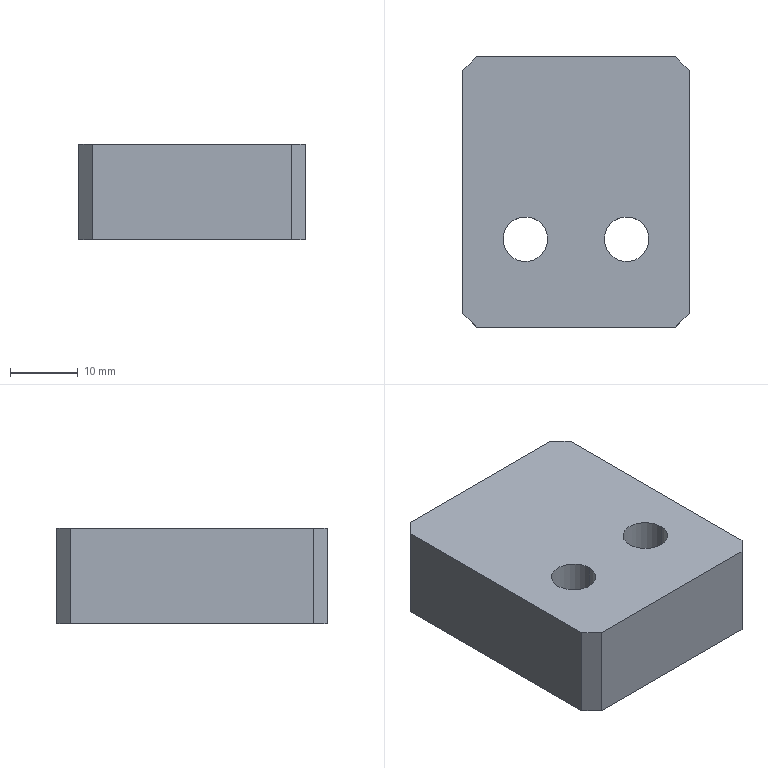Part | NX | features BREP 1 | 1 solid | 28 faces | box 33.5 x 40 x 14.15 mm | volume 16795 mm3 | cylinder 12 | plane 12 | cone 4 | commonest cylinder face diameters 4.2 x4 6.6 x4 11 x4
STEP:
#1=CARTESIAN_POINT('',(14.,-31.,6.));
#2=VERTEX_POINT('',#1);
#3=CARTESIAN_POINT('',(3.,-31.,6.));
#4=VERTEX_POINT('',#3);
#5=CARTESIAN_POINT('',(8.5,-31.,6.));
#6=DIRECTION('',(0.,0.,-1.));
#7=DIRECTION('',(-1.,0.,0.));
#8=AXIS2_PLACEMENT_3D('',#5,#6,#7);
#9=CIRCLE('',#8,5.5);
#10=EDGE_CURVE('',#2,#4,#9,.T.);
#11=ORIENTED_EDGE('',*,*,#10,.F.);
#12=CARTESIAN_POINT('',(14.,-31.,0.));
#13=VERTEX_POINT('',#12);
#14=CARTESIAN_POINT('',(14.,-31.,0.));
#15=DIRECTION('',(0.,0.,-1.));
#16=VECTOR('',#15,1000.);
#17=LINE('',#14,#16);
#18=EDGE_CURVE('',#2,#13,#17,.T.);
#19=ORIENTED_EDGE('',*,*,#18,.T.);
#20=CARTESIAN_POINT('',(3.,-31.,0.));
#21=VERTEX_POINT('',#20);
#22=CARTESIAN_POINT('',(8.5,-31.,0.));
#23=DIRECTION('',(0.,0.,-1.));
#24=DIRECTION('',(-1.,0.,0.));
#25=AXIS2_PLACEMENT_3D('',#22,#23,#24);
#26=CIRCLE('',#25,5.5);
#27=EDGE_CURVE('',#13,#21,#26,.T.);
#28=ORIENTED_EDGE('',*,*,#27,.T.);
#29=CARTESIAN_POINT('',(3.,-31.,0.));
#30=DIRECTION('',(0.,0.,-1.));
#31=VECTOR('',#30,1000.);
#32=LINE('',#29,#31);
#33=EDGE_CURVE('',#4,#21,#32,.T.);
#34=ORIENTED_EDGE('',*,*,#33,.F.);
#35=EDGE_LOOP('',(#11,#19,#28,#34));
#36=FACE_BOUND('',#35,.T.);
#37=CARTESIAN_POINT('',(8.5,-31.,0.));
#38=DIRECTION('',(0.,0.,-1.));
#39=DIRECTION('',(-1.,0.,0.));
#40=AXIS2_PLACEMENT_3D('',#37,#38,#39);
#41=CYLINDRICAL_SURFACE('',#40,5.5);
#42=ADVANCED_FACE('',(#36),#41,.F.);
#43=CARTESIAN_POINT('',(11.8,-31.,14.15));
#44=VERTEX_POINT('',#43);
#45=CARTESIAN_POINT('',(5.2,-31.,14.15));
#46=VERTEX_POINT('',#45);
#47=CARTESIAN_POINT('',(8.5,-31.,14.15));
#48=DIRECTION('',(0.,0.,-1.));
#49=DIRECTION('',(-1.,0.,0.));
#50=AXIS2_PLACEMENT_3D('',#47,#48,#49);
#51=CIRCLE('',#50,3.3);
#52=EDGE_CURVE('',#44,#46,#51,.T.);
#53=ORIENTED_EDGE('',*,*,#52,.F.);
#54=CARTESIAN_POINT('',(11.8,-31.,6.));
#55=VERTEX_POINT('',#54);
#56=CARTESIAN_POINT('',(11.8,-31.,0.));
#57=DIRECTION('',(0.,0.,-1.));
#58=VECTOR('',#57,1000.);
#59=LINE('',#56,#58);
#60=EDGE_CURVE('',#44,#55,#59,.T.);
#61=ORIENTED_EDGE('',*,*,#60,.T.);
#62=CARTESIAN_POINT('',(5.2,-31.,6.));
#63=VERTEX_POINT('',#62);
#64=CARTESIAN_POINT('',(8.5,-31.,6.));
#65=DIRECTION('',(0.,0.,-1.));
#66=DIRECTION('',(-1.,0.,0.));
#67=AXIS2_PLACEMENT_3D('',#64,#65,#66);
#68=CIRCLE('',#67,3.3);
#69=EDGE_CURVE('',#55,#63,#68,.T.);
#70=ORIENTED_EDGE('',*,*,#69,.T.);
#71=CARTESIAN_POINT('',(5.2,-31.,0.));
#72=DIRECTION('',(0.,0.,-1.));
#73=VECTOR('',#72,1000.);
#74=LINE('',#71,#73);
#75=EDGE_CURVE('',#46,#63,#74,.T.);
#76=ORIENTED_EDGE('',*,*,#75,.F.);
#77=EDGE_LOOP('',(#53,#61,#70,#76));
#78=FACE_BOUND('',#77,.T.);
#79=CARTESIAN_POINT('',(8.5,-31.,0.));
#80=DIRECTION('',(0.,0.,-1.));
#81=DIRECTION('',(-1.,0.,0.));
#82=AXIS2_PLACEMENT_3D('',#79,#80,#81);
#83=CYLINDRICAL_SURFACE('',#82,3.3);
#84=ADVANCED_FACE('',(#78),#83,.F.);
#85=CARTESIAN_POINT('',(-1.,-31.,6.));
#86=VERTEX_POINT('',#85);
#87=CARTESIAN_POINT('',(-12.,-31.,6.));
#88=VERTEX_POINT('',#87);
#89=CARTESIAN_POINT('',(-6.5,-31.,6.));
#90=DIRECTION('',(0.,0.,-1.));
#91=DIRECTION('',(-1.,0.,0.));
#92=AXIS2_PLACEMENT_3D('',#89,#90,#91);
#93=CIRCLE('',#92,5.5);
#94=EDGE_CURVE('',#86,#88,#93,.T.);
#95=ORIENTED_EDGE('',*,*,#94,.F.);
#96=CARTESIAN_POINT('',(-1.,-31.,0.));
#97=VERTEX_POINT('',#96);
#98=CARTESIAN_POINT('',(-1.,-31.,0.));
#99=DIRECTION('',(0.,0.,-1.));
#100=VECTOR('',#99,1000.);
#101=LINE('',#98,#100);
#102=EDGE_CURVE('',#86,#97,#101,.T.);
#103=ORIENTED_EDGE('',*,*,#102,.T.);
#104=CARTESIAN_POINT('',(-12.,-31.,0.));
#105=VERTEX_POINT('',#104);
#106=CARTESIAN_POINT('',(-6.5,-31.,0.));
#107=DIRECTION('',(0.,0.,-1.));
#108=DIRECTION('',(-1.,0.,0.));
#109=AXIS2_PLACEMENT_3D('',#106,#107,#108);
#110=CIRCLE('',#109,5.5);
#111=EDGE_CURVE('',#97,#105,#110,.T.);
#112=ORIENTED_EDGE('',*,*,#111,.T.);
#113=CARTESIAN_POINT('',(-12.,-31.,0.));
#114=DIRECTION('',(0.,0.,-1.));
#115=VECTOR('',#114,1000.);
#116=LINE('',#113,#115);
#117=EDGE_CURVE('',#88,#105,#116,.T.);
#118=ORIENTED_EDGE('',*,*,#117,.F.);
#119=EDGE_LOOP('',(#95,#103,#112,#118));
#120=FACE_BOUND('',#119,.T.);
#121=CARTESIAN_POINT('',(-6.5,-31.,0.));
#122=DIRECTION('',(0.,0.,-1.));
#123=DIRECTION('',(-1.,0.,0.));
#124=AXIS2_PLACEMENT_3D('',#121,#122,#123);
#125=CYLINDRICAL_SURFACE('',#124,5.5);
#126=ADVANCED_FACE('',(#120),#125,.F.);
#127=CARTESIAN_POINT('',(-3.2,-31.,14.15));
#128=VERTEX_POINT('',#127);
#129=CARTESIAN_POINT('',(-9.8,-31.,14.15));
#130=VERTEX_POINT('',#129);
#131=CARTESIAN_POINT('',(-6.5,-31.,14.15));
#132=DIRECTION('',(0.,0.,-1.));
#133=DIRECTION('',(-1.,0.,0.));
#134=AXIS2_PLACEMENT_3D('',#131,#132,#133);
#135=CIRCLE('',#134,3.3);
#136=EDGE_CURVE('',#128,#130,#135,.T.);
#137=ORIENTED_EDGE('',*,*,#136,.F.);
#138=CARTESIAN_POINT('',(-3.2,-31.,6.));
#139=VERTEX_POINT('',#138);
#140=CARTESIAN_POINT('',(-3.2,-31.,0.));
#141=DIRECTION('',(0.,0.,-1.));
#142=VECTOR('',#141,1000.);
#143=LINE('',#140,#142);
#144=EDGE_CURVE('',#128,#139,#143,.T.);
#145=ORIENTED_EDGE('',*,*,#144,.T.);
#146=CARTESIAN_POINT('',(-9.8,-31.,6.));
#147=VERTEX_POINT('',#146);
#148=CARTESIAN_POINT('',(-6.5,-31.,6.));
#149=DIRECTION('',(0.,0.,-1.));
#150=DIRECTION('',(-1.,0.,0.));
#151=AXIS2_PLACEMENT_3D('',#148,#149,#150);
#152=CIRCLE('',#151,3.3);
#153=EDGE_CURVE('',#139,#147,#152,.T.);
#154=ORIENTED_EDGE('',*,*,#153,.T.);
#155=CARTESIAN_POINT('',(-9.8,-31.,0.));
#156=DIRECTION('',(0.,0.,-1.));
#157=VECTOR('',#156,1000.);
#158=LINE('',#155,#157);
#159=EDGE_CURVE('',#130,#147,#158,.T.);
#160=ORIENTED_EDGE('',*,*,#159,.F.);
#161=EDGE_LOOP('',(#137,#145,#154,#160));
#162=FACE_BOUND('',#161,.T.);
#163=CARTESIAN_POINT('',(-6.5,-31.,0.));
#164=DIRECTION('',(0.,0.,-1.));
#165=DIRECTION('',(-1.,0.,0.));
#166=AXIS2_PLACEMENT_3D('',#163,#164,#165);
#167=CYLINDRICAL_SURFACE('',#166,3.3);
#168=ADVANCED_FACE('',(#162),#167,.F.);
#169=CARTESIAN_POINT('',(13.6,-16.,12.4));
#170=VERTEX_POINT('',#169);
#171=CARTESIAN_POINT('',(9.4,-16.,12.4));
#172=VERTEX_POINT('',#171);
#173=CARTESIAN_POINT('',(11.5,-16.,12.4));
#174=DIRECTION('',(0.,0.,-1.));
#175=DIRECTION('',(-1.,0.,0.));
#176=AXIS2_PLACEMENT_3D('',#173,#174,#175);
#177=CIRCLE('',#176,2.1);
#178=EDGE_CURVE('',#170,#172,#177,.T.);
#179=ORIENTED_EDGE('',*,*,#178,.F.);
#180=CARTESIAN_POINT('',(13.6,-16.,0.));
#181=VERTEX_POINT('',#180);
#182=CARTESIAN_POINT('',(13.6,-16.,0.));
#183=DIRECTION('',(0.,0.,-1.));
#184=VECTOR('',#183,1000.);
#185=LINE('',#182,#184);
#186=EDGE_CURVE('',#170,#181,#185,.T.);
#187=ORIENTED_EDGE('',*,*,#186,.T.);
#188=CARTESIAN_POINT('',(9.4,-16.,0.));
#189=VERTEX_POINT('',#188);
#190=CARTESIAN_POINT('',(11.5,-16.,0.));
#191=DIRECTION('',(0.,0.,-1.));
#192=DIRECTION('',(-1.,0.,0.));
#193=AXIS2_PLACEMENT_3D('',#190,#191,#192);
#194=CIRCLE('',#193,2.1);
#195=EDGE_CURVE('',#181,#189,#194,.T.);
#196=ORIENTED_EDGE('',*,*,#195,.T.);
#197=CARTESIAN_POINT('',(9.4,-16.,0.));
#198=DIRECTION('',(0.,0.,-1.));
#199=VECTOR('',#198,1000.);
#200=LINE('',#197,#199);
#201=EDGE_CURVE('',#172,#189,#200,.T.);
#202=ORIENTED_EDGE('',*,*,#201,.F.);
#203=EDGE_LOOP('',(#179,#187,#196,#202));
#204=FACE_BOUND('',#203,.T.);
#205=CARTESIAN_POINT('',(11.5,-16.,0.));
#206=DIRECTION('',(0.,0.,-1.));
#207=DIRECTION('',(-1.,0.,0.));
#208=AXIS2_PLACEMENT_3D('',#205,#206,#207);
#209=CYLINDRICAL_SURFACE('',#208,2.1);
#210=ADVANCED_FACE('',(#204),#209,.F.);
#211=CARTESIAN_POINT('',(11.5,-16.,13.662));
#212=VERTEX_POINT('',#211);
#213=CARTESIAN_POINT('',(9.4,-16.,12.4));
#214=DIRECTION('',(-0.8572,0.,-0.515));
#215=VECTOR('',#214,1000.);
#216=LINE('',#213,#215);
#217=EDGE_CURVE('',#212,#172,#216,.T.);
#218=ORIENTED_EDGE('',*,*,#217,.F.);
#219=CARTESIAN_POINT('',(13.6,-16.,12.4));
#220=DIRECTION('',(0.8572,0.,-0.515));
#221=VECTOR('',#220,1000.);
#222=LINE('',#219,#221);
#223=EDGE_CURVE('',#212,#170,#222,.T.);
#224=ORIENTED_EDGE('',*,*,#223,.T.);
#225=ORIENTED_EDGE('',*,*,#178,.T.);
#226=EDGE_LOOP('',(#218,#224,#225));
#227=FACE_BOUND('',#226,.T.);
#228=CARTESIAN_POINT('',(11.5,-16.,12.4));
#229=DIRECTION('',(0.,0.,-1.));
#230=DIRECTION('',(-1.,0.,0.));
#231=AXIS2_PLACEMENT_3D('',#228,#229,#230);
#232=CONICAL_SURFACE('',#231,2.1,1.03);
#233=ADVANCED_FACE('',(#227),#232,.F.);
#234=CARTESIAN_POINT('',(-7.4,-16.,12.4));
#235=VERTEX_POINT('',#234);
#236=CARTESIAN_POINT('',(-11.6,-16.,12.4));
#237=VERTEX_POINT('',#236);
#238=CARTESIAN_POINT('',(-9.5,-16.,12.4));
#239=DIRECTION('',(0.,0.,-1.));
#240=DIRECTION('',(-1.,0.,0.));
#241=AXIS2_PLACEMENT_3D('',#238,#239,#240);
#242=CIRCLE('',#241,2.1);
#243=EDGE_CURVE('',#235,#237,#242,.T.);
#244=ORIENTED_EDGE('',*,*,#243,.F.);
#245=CARTESIAN_POINT('',(-7.4,-16.,0.));
#246=VERTEX_POINT('',#245);
#247=CARTESIAN_POINT('',(-7.4,-16.,0.));
#248=DIRECTION('',(0.,0.,-1.));
#249=VECTOR('',#248,1000.);
#250=LINE('',#247,#249);
#251=EDGE_CURVE('',#235,#246,#250,.T.);
#252=ORIENTED_EDGE('',*,*,#251,.T.);
#253=CARTESIAN_POINT('',(-11.6,-16.,0.));
#254=VERTEX_POINT('',#253);
#255=CARTESIAN_POINT('',(-9.5,-16.,0.));
#256=DIRECTION('',(0.,0.,-1.));
#257=DIRECTION('',(-1.,0.,0.));
#258=AXIS2_PLACEMENT_3D('',#255,#256,#257);
#259=CIRCLE('',#258,2.1);
#260=EDGE_CURVE('',#246,#254,#259,.T.);
#261=ORIENTED_EDGE('',*,*,#260,.T.);
#262=CARTESIAN_POINT('',(-11.6,-16.,0.));
#263=DIRECTION('',(0.,0.,-1.));
#264=VECTOR('',#263,1000.);
#265=LINE('',#262,#264);
#266=EDGE_CURVE('',#237,#254,#265,.T.);
#267=ORIENTED_EDGE('',*,*,#266,.F.);
#268=EDGE_LOOP('',(#244,#252,#261,#267));
#269=FACE_BOUND('',#268,.T.);
#270=CARTESIAN_POINT('',(-9.5,-16.,0.));
#271=DIRECTION('',(0.,0.,-1.));
#272=DIRECTION('',(-1.,0.,0.));
#273=AXIS2_PLACEMENT_3D('',#270,#271,#272);
#274=CYLINDRICAL_SURFACE('',#273,2.1);
#275=ADVANCED_FACE('',(#269),#274,.F.);
#276=CARTESIAN_POINT('',(-9.5,-16.,13.662));
#277=VERTEX_POINT('',#276);
#278=CARTESIAN_POINT('',(-11.6,-16.,12.4));
#279=DIRECTION('',(-0.8572,0.,-0.515));
#280=VECTOR('',#279,1000.);
#281=LINE('',#278,#280);
#282=EDGE_CURVE('',#277,#237,#281,.T.);
#283=ORIENTED_EDGE('',*,*,#282,.F.);
#284=CARTESIAN_POINT('',(-7.4,-16.,12.4));
#285=DIRECTION('',(0.8572,0.,-0.515));
#286=VECTOR('',#285,1000.);
#287=LINE('',#284,#286);
#288=EDGE_CURVE('',#277,#235,#287,.T.);
#289=ORIENTED_EDGE('',*,*,#288,.T.);
#290=ORIENTED_EDGE('',*,*,#243,.T.);
#291=EDGE_LOOP('',(#283,#289,#290));
#292=FACE_BOUND('',#291,.T.);
#293=CARTESIAN_POINT('',(-9.5,-16.,12.4));
#294=DIRECTION('',(0.,0.,-1.));
#295=DIRECTION('',(-1.,0.,0.));
#296=AXIS2_PLACEMENT_3D('',#293,#294,#295);
#297=CONICAL_SURFACE('',#296,2.1,1.03);
#298=ADVANCED_FACE('',(#292),#297,.F.);
#299=CARTESIAN_POINT('',(-15.75,-6.,14.15));
#300=VERTEX_POINT('',#299);
#301=CARTESIAN_POINT('',(-15.75,-42.,14.15));
#302=VERTEX_POINT('',#301);
#303=CARTESIAN_POINT('',(-15.75,-4.,14.15));
#304=DIRECTION('',(0.,-1.,0.));
#305=VECTOR('',#304,1000.);
#306=LINE('',#303,#305);
#307=EDGE_CURVE('',#300,#302,#306,.T.);
#308=ORIENTED_EDGE('',*,*,#307,.F.);
#309=CARTESIAN_POINT('',(-15.75,-6.,0.));
#310=VERTEX_POINT('',#309);
#311=CARTESIAN_POINT('',(-15.75,-6.,14.15));
#312=DIRECTION('',(0.,0.,-1.));
#313=VECTOR('',#312,1000.);
#314=LINE('',#311,#313);
#315=EDGE_CURVE('',#300,#310,#314,.T.);
#316=ORIENTED_EDGE('',*,*,#315,.T.);
#317=CARTESIAN_POINT('',(-15.75,-42.,0.));
#318=VERTEX_POINT('',#317);
#319=CARTESIAN_POINT('',(-15.75,-4.,0.));
#320=DIRECTION('',(0.,-1.,0.));
#321=VECTOR('',#320,1000.);
#322=LINE('',#319,#321);
#323=EDGE_CURVE('',#310,#318,#322,.T.);
#324=ORIENTED_EDGE('',*,*,#323,.T.);
#325=CARTESIAN_POINT('',(-15.75,-42.,14.15));
#326=DIRECTION('',(0.,0.,1.));
#327=VECTOR('',#326,1000.);
#328=LINE('',#325,#327);
#329=EDGE_CURVE('',#318,#302,#328,.T.);
#330=ORIENTED_EDGE('',*,*,#329,.T.);
#331=EDGE_LOOP('',(#308,#316,#324,#330));
#332=FACE_BOUND('',#331,.T.);
#333=CARTESIAN_POINT('',(-15.75,-4.,14.15));
#334=DIRECTION('',(1.,0.,0.));
#335=DIRECTION('',(0.,-1.,0.));
#336=AXIS2_PLACEMENT_3D('',#333,#334,#335);
#337=PLANE('',#336);
#338=ADVANCED_FACE('',(#332),#337,.F.);
#339=CARTESIAN_POINT('',(-13.75,-44.,0.));
#340=VERTEX_POINT('',#339);
#341=CARTESIAN_POINT('',(15.75,-44.,0.));
#342=VERTEX_POINT('',#341);
#343=CARTESIAN_POINT('',(-15.75,-44.,0.));
#344=DIRECTION('',(1.,0.,0.));
#345=VECTOR('',#344,1000.);
#346=LINE('',#343,#345);
#347=EDGE_CURVE('',#340,#342,#346,.T.);
#348=ORIENTED_EDGE('',*,*,#347,.T.);
#349=CARTESIAN_POINT('',(15.75,-44.,14.15));
#350=VERTEX_POINT('',#349);
#351=CARTESIAN_POINT('',(15.75,-44.,14.15));
#352=DIRECTION('',(0.,0.,1.));
#353=VECTOR('',#352,1000.);
#354=LINE('',#351,#353);
#355=EDGE_CURVE('',#342,#350,#354,.T.);
#356=ORIENTED_EDGE('',*,*,#355,.T.);
#357=CARTESIAN_POINT('',(-13.75,-44.,14.15));
#358=VERTEX_POINT('',#357);
#359=CARTESIAN_POINT('',(-15.75,-44.,14.15));
#360=DIRECTION('',(1.,0.,0.));
#361=VECTOR('',#360,1000.);
#362=LINE('',#359,#361);
#363=EDGE_CURVE('',#358,#350,#362,.T.);
#364=ORIENTED_EDGE('',*,*,#363,.F.);
#365=CARTESIAN_POINT('',(-13.75,-44.,14.15));
#366=DIRECTION('',(0.,0.,-1.));
#367=VECTOR('',#366,1000.);
#368=LINE('',#365,#367);
#369=EDGE_CURVE('',#358,#340,#368,.T.);
#370=ORIENTED_EDGE('',*,*,#369,.T.);
#371=EDGE_LOOP('',(#348,#356,#364,#370));
#372=FACE_BOUND('',#371,.T.);
#373=CARTESIAN_POINT('',(-15.75,-44.,14.15));
#374=DIRECTION('',(0.,1.,0.));
#375=DIRECTION('',(1.,0.,0.));
#376=AXIS2_PLACEMENT_3D('',#373,#374,#375);
#377=PLANE('',#376);
#378=ADVANCED_FACE('',(#372),#377,.F.);
#379=CARTESIAN_POINT('',(17.75,-42.,14.15));
#380=VERTEX_POINT('',#379);
#381=CARTESIAN_POINT('',(17.75,-6.,14.15));
#382=VERTEX_POINT('',#381);
#383=CARTESIAN_POINT('',(17.75,-4.,14.15));
#384=DIRECTION('',(0.,1.,0.));
#385=VECTOR('',#384,1000.);
#386=LINE('',#383,#385);
#387=EDGE_CURVE('',#380,#382,#386,.T.);
#388=ORIENTED_EDGE('',*,*,#387,.F.);
#389=CARTESIAN_POINT('',(17.75,-42.,0.));
#390=VERTEX_POINT('',#389);
#391=CARTESIAN_POINT('',(17.75,-42.,14.15));
#392=DIRECTION('',(0.,0.,-1.));
#393=VECTOR('',#392,1000.);
#394=LINE('',#391,#393);
#395=EDGE_CURVE('',#380,#390,#394,.T.);
#396=ORIENTED_EDGE('',*,*,#395,.T.);
#397=CARTESIAN_POINT('',(17.75,-6.,0.));
#398=VERTEX_POINT('',#397);
#399=CARTESIAN_POINT('',(17.75,-4.,0.));
#400=DIRECTION('',(0.,1.,0.));
#401=VECTOR('',#400,1000.);
#402=LINE('',#399,#401);
#403=EDGE_CURVE('',#390,#398,#402,.T.);
#404=ORIENTED_EDGE('',*,*,#403,.T.);
#405=CARTESIAN_POINT('',(17.75,-6.,14.15));
#406=DIRECTION('',(0.,0.,1.));
#407=VECTOR('',#406,1000.);
#408=LINE('',#405,#407);
#409=EDGE_CURVE('',#398,#382,#408,.T.);
#410=ORIENTED_EDGE('',*,*,#409,.T.);
#411=EDGE_LOOP('',(#388,#396,#404,#410));
#412=FACE_BOUND('',#411,.T.);
#413=CARTESIAN_POINT('',(17.75,-4.,14.15));
#414=DIRECTION('',(-1.,0.,0.));
#415=DIRECTION('',(0.,1.,0.));
#416=AXIS2_PLACEMENT_3D('',#413,#414,#415);
#417=PLANE('',#416);
#418=ADVANCED_FACE('',(#412),#417,.F.);
#419=CARTESIAN_POINT('',(15.75,-4.,14.15));
#420=VERTEX_POINT('',#419);
#421=CARTESIAN_POINT('',(-13.75,-4.,14.15));
#422=VERTEX_POINT('',#421);
#423=CARTESIAN_POINT('',(-15.75,-4.,14.15));
#424=DIRECTION('',(-1.,0.,0.));
#425=VECTOR('',#424,1000.);
#426=LINE('',#423,#425);
#427=EDGE_CURVE('',#420,#422,#426,.T.);
#428=ORIENTED_EDGE('',*,*,#427,.F.);
#429=CARTESIAN_POINT('',(15.75,-4.,0.));
#430=VERTEX_POINT('',#429);
#431=CARTESIAN_POINT('',(15.75,-4.,14.15));
#432=DIRECTION('',(0.,0.,-1.));
#433=VECTOR('',#432,1000.);
#434=LINE('',#431,#433);
#435=EDGE_CURVE('',#420,#430,#434,.T.);
#436=ORIENTED_EDGE('',*,*,#435,.T.);
#437=CARTESIAN_POINT('',(-13.75,-4.,0.));
#438=VERTEX_POINT('',#437);
#439=CARTESIAN_POINT('',(-15.75,-4.,0.));
#440=DIRECTION('',(-1.,0.,0.));
#441=VECTOR('',#440,1000.);
#442=LINE('',#439,#441);
#443=EDGE_CURVE('',#430,#438,#442,.T.);
#444=ORIENTED_EDGE('',*,*,#443,.T.);
#445=CARTESIAN_POINT('',(-13.75,-4.,14.15));
#446=DIRECTION('',(0.,0.,1.));
#447=VECTOR('',#446,1000.);
#448=LINE('',#445,#447);
#449=EDGE_CURVE('',#438,#422,#448,.T.);
#450=ORIENTED_EDGE('',*,*,#449,.T.);
#451=EDGE_LOOP('',(#428,#436,#444,#450));
#452=FACE_BOUND('',#451,.T.);
#453=CARTESIAN_POINT('',(-15.75,-4.,14.15));
#454=DIRECTION('',(0.,-1.,0.));
#455=DIRECTION('',(0.,0.,-1.));
#456=AXIS2_PLACEMENT_3D('',#453,#454,#455);
#457=PLANE('',#456);
#458=ADVANCED_FACE('',(#452),#457,.F.);
#459=ORIENTED_EDGE('',*,*,#363,.T.);
#460=CARTESIAN_POINT('',(0.,-59.75,14.15));
#461=DIRECTION('',(0.7071,0.7071,0.));
#462=VECTOR('',#461,1000.);
#463=LINE('',#460,#462);
#464=EDGE_CURVE('',#350,#380,#463,.T.);
#465=ORIENTED_EDGE('',*,*,#464,.T.);
#466=ORIENTED_EDGE('',*,*,#387,.T.);
#467=CARTESIAN_POINT('',(20.,-8.25,14.15));
#468=DIRECTION('',(-0.7071,0.7071,0.));
#469=VECTOR('',#468,1000.);
#470=LINE('',#467,#469);
#471=EDGE_CURVE('',#382,#420,#470,.T.);
#472=ORIENTED_EDGE('',*,*,#471,.T.);
#473=ORIENTED_EDGE('',*,*,#427,.T.);
#474=CARTESIAN_POINT('',(-34.75,-25.,14.15));
#475=DIRECTION('',(-0.7071,-0.7071,0.));
#476=VECTOR('',#475,1000.);
#477=LINE('',#474,#476);
#478=EDGE_CURVE('',#422,#300,#477,.T.);
#479=ORIENTED_EDGE('',*,*,#478,.T.);
#480=ORIENTED_EDGE('',*,*,#307,.T.);
#481=CARTESIAN_POINT('',(-14.75,-43.,14.15));
#482=DIRECTION('',(0.7071,-0.7071,0.));
#483=VECTOR('',#482,1000.);
#484=LINE('',#481,#483);
#485=EDGE_CURVE('',#302,#358,#484,.T.);
#486=ORIENTED_EDGE('',*,*,#485,.T.);
#487=EDGE_LOOP('',(#459,#465,#466,#472,#473,#479,#480,#486));
#488=FACE_BOUND('',#487,.T.);
#489=CARTESIAN_POINT('',(8.5,-31.,14.15));
#490=DIRECTION('',(0.,0.,-1.));
#491=DIRECTION('',(-1.,0.,0.));
#492=AXIS2_PLACEMENT_3D('',#489,#490,#491);
#493=CIRCLE('',#492,3.3);
#494=EDGE_CURVE('',#46,#44,#493,.T.);
#495=ORIENTED_EDGE('',*,*,#494,.T.);
#496=ORIENTED_EDGE('',*,*,#52,.T.);
#497=EDGE_LOOP('',(#495,#496));
#498=FACE_BOUND('',#497,.T.);
#499=CARTESIAN_POINT('',(-6.5,-31.,14.15));
#500=DIRECTION('',(0.,0.,-1.));
#501=DIRECTION('',(-1.,0.,0.));
#502=AXIS2_PLACEMENT_3D('',#499,#500,#501);
#503=CIRCLE('',#502,3.3);
#504=EDGE_CURVE('',#130,#128,#503,.T.);
#505=ORIENTED_EDGE('',*,*,#504,.T.);
#506=ORIENTED_EDGE('',*,*,#136,.T.);
#507=EDGE_LOOP('',(#505,#506));
#508=FACE_BOUND('',#507,.T.);
#509=CARTESIAN_POINT('',(-15.75,-44.,14.15));
#510=DIRECTION('',(0.,0.,1.));
#511=DIRECTION('',(1.,0.,0.));
#512=AXIS2_PLACEMENT_3D('',#509,#510,#511);
#513=PLANE('',#512);
#514=ADVANCED_FACE('',(#488,#498,#508),#513,.T.);
#515=ORIENTED_EDGE('',*,*,#403,.F.);
#516=CARTESIAN_POINT('',(17.75,-42.,0.));
#517=DIRECTION('',(-0.7071,-0.7071,0.));
#518=VECTOR('',#517,1000.);
#519=LINE('',#516,#518);
#520=EDGE_CURVE('',#390,#342,#519,.T.);
#521=ORIENTED_EDGE('',*,*,#520,.T.);
#522=ORIENTED_EDGE('',*,*,#347,.F.);
#523=CARTESIAN_POINT('',(-13.75,-44.,0.));
#524=DIRECTION('',(-0.7071,0.7071,0.));
#525=VECTOR('',#524,1000.);
#526=LINE('',#523,#525);
#527=EDGE_CURVE('',#340,#318,#526,.T.);
#528=ORIENTED_EDGE('',*,*,#527,.T.);
#529=ORIENTED_EDGE('',*,*,#323,.F.);
#530=CARTESIAN_POINT('',(-15.75,-6.,0.));
#531=DIRECTION('',(0.7071,0.7071,0.));
#532=VECTOR('',#531,1000.);
#533=LINE('',#530,#532);
#534=EDGE_CURVE('',#310,#438,#533,.T.);
#535=ORIENTED_EDGE('',*,*,#534,.T.);
#536=ORIENTED_EDGE('',*,*,#443,.F.);
#537=CARTESIAN_POINT('',(15.75,-4.,0.));
#538=DIRECTION('',(0.7071,-0.7071,0.));
#539=VECTOR('',#538,1000.);
#540=LINE('',#537,#539);
#541=EDGE_CURVE('',#430,#398,#540,.T.);
#542=ORIENTED_EDGE('',*,*,#541,.T.);
#543=EDGE_LOOP('',(#515,#521,#522,#528,#529,#535,#536,#542));
#544=FACE_BOUND('',#543,.T.);
#545=CARTESIAN_POINT('',(8.5,-31.,0.));
#546=DIRECTION('',(0.,0.,-1.));
#547=DIRECTION('',(-1.,0.,0.));
#548=AXIS2_PLACEMENT_3D('',#545,#546,#547);
#549=CIRCLE('',#548,5.5);
#550=EDGE_CURVE('',#21,#13,#549,.T.);
#551=ORIENTED_EDGE('',*,*,#550,.F.);
#552=ORIENTED_EDGE('',*,*,#27,.F.);
#553=EDGE_LOOP('',(#551,#552));
#554=FACE_BOUND('',#553,.T.);
#555=CARTESIAN_POINT('',(-6.5,-31.,0.));
#556=DIRECTION('',(0.,0.,-1.));
#557=DIRECTION('',(-1.,0.,0.));
#558=AXIS2_PLACEMENT_3D('',#555,#556,#557);
#559=CIRCLE('',#558,5.5);
#560=EDGE_CURVE('',#105,#97,#559,.T.);
#561=ORIENTED_EDGE('',*,*,#560,.F.);
#562=ORIENTED_EDGE('',*,*,#111,.F.);
#563=EDGE_LOOP('',(#561,#562));
#564=FACE_BOUND('',#563,.T.);
#565=CARTESIAN_POINT('',(11.5,-16.,0.));
#566=DIRECTION('',(0.,0.,-1.));
#567=DIRECTION('',(-1.,0.,0.));
#568=AXIS2_PLACEMENT_3D('',#565,#566,#567);
#569=CIRCLE('',#568,2.1);
#570=EDGE_CURVE('',#189,#181,#569,.T.);
#571=ORIENTED_EDGE('',*,*,#570,.F.);
#572=ORIENTED_EDGE('',*,*,#195,.F.);
#573=EDGE_LOOP('',(#571,#572));
#574=FACE_BOUND('',#573,.T.);
#575=CARTESIAN_POINT('',(-9.5,-16.,0.));
#576=DIRECTION('',(0.,0.,-1.));
#577=DIRECTION('',(-1.,0.,0.));
#578=AXIS2_PLACEMENT_3D('',#575,#576,#577);
#579=CIRCLE('',#578,2.1);
#580=EDGE_CURVE('',#254,#246,#579,.T.);
#581=ORIENTED_EDGE('',*,*,#580,.F.);
#582=ORIENTED_EDGE('',*,*,#260,.F.);
#583=EDGE_LOOP('',(#581,#582));
#584=FACE_BOUND('',#583,.T.);
#585=CARTESIAN_POINT('',(-15.75,-44.,0.));
#586=DIRECTION('',(0.,0.,1.));
#587=DIRECTION('',(1.,0.,0.));
#588=AXIS2_PLACEMENT_3D('',#585,#586,#587);
#589=PLANE('',#588);
#590=ADVANCED_FACE('',(#544,#554,#564,#574,#584),#589,.F.);
#591=ORIENTED_EDGE('',*,*,#288,.F.);
#592=ORIENTED_EDGE('',*,*,#282,.T.);
#593=CARTESIAN_POINT('',(-9.5,-16.,12.4));
#594=DIRECTION('',(0.,0.,-1.));
#595=DIRECTION('',(-1.,0.,0.));
#596=AXIS2_PLACEMENT_3D('',#593,#594,#595);
#597=CIRCLE('',#596,2.1);
#598=EDGE_CURVE('',#237,#235,#597,.T.);
#599=ORIENTED_EDGE('',*,*,#598,.T.);
#600=EDGE_LOOP('',(#591,#592,#599));
#601=FACE_BOUND('',#600,.T.);
#602=CARTESIAN_POINT('',(-9.5,-16.,12.4));
#603=DIRECTION('',(0.,0.,-1.));
#604=DIRECTION('',(-1.,0.,0.));
#605=AXIS2_PLACEMENT_3D('',#602,#603,#604);
#606=CONICAL_SURFACE('',#605,2.1,1.03);
#607=ADVANCED_FACE('',(#601),#606,.F.);
#608=ORIENTED_EDGE('',*,*,#251,.F.);
#609=ORIENTED_EDGE('',*,*,#598,.F.);
#610=ORIENTED_EDGE('',*,*,#266,.T.);
#611=ORIENTED_EDGE('',*,*,#580,.T.);
#612=EDGE_LOOP('',(#608,#609,#610,#611));
#613=FACE_BOUND('',#612,.T.);
#614=CARTESIAN_POINT('',(-9.5,-16.,0.));
#615=DIRECTION('',(0.,0.,-1.));
#616=DIRECTION('',(-1.,0.,0.));
#617=AXIS2_PLACEMENT_3D('',#614,#615,#616);
#618=CYLINDRICAL_SURFACE('',#617,2.1);
#619=ADVANCED_FACE('',(#613),#618,.F.);
#620=ORIENTED_EDGE('',*,*,#223,.F.);
#621=ORIENTED_EDGE('',*,*,#217,.T.);
#622=CARTESIAN_POINT('',(11.5,-16.,12.4));
#623=DIRECTION('',(0.,0.,-1.));
#624=DIRECTION('',(-1.,0.,0.));
#625=AXIS2_PLACEMENT_3D('',#622,#623,#624);
#626=CIRCLE('',#625,2.1);
#627=EDGE_CURVE('',#172,#170,#626,.T.);
#628=ORIENTED_EDGE('',*,*,#627,.T.);
#629=EDGE_LOOP('',(#620,#621,#628));
#630=FACE_BOUND('',#629,.T.);
#631=CARTESIAN_POINT('',(11.5,-16.,12.4));
#632=DIRECTION('',(0.,0.,-1.));
#633=DIRECTION('',(-1.,0.,0.));
#634=AXIS2_PLACEMENT_3D('',#631,#632,#633);
#635=CONICAL_SURFACE('',#634,2.1,1.03);
#636=ADVANCED_FACE('',(#630),#635,.F.);
#637=ORIENTED_EDGE('',*,*,#186,.F.);
#638=ORIENTED_EDGE('',*,*,#627,.F.);
#639=ORIENTED_EDGE('',*,*,#201,.T.);
#640=ORIENTED_EDGE('',*,*,#570,.T.);
#641=EDGE_LOOP('',(#637,#638,#639,#640));
#642=FACE_BOUND('',#641,.T.);
#643=CARTESIAN_POINT('',(11.5,-16.,0.));
#644=DIRECTION('',(0.,0.,-1.));
#645=DIRECTION('',(-1.,0.,0.));
#646=AXIS2_PLACEMENT_3D('',#643,#644,#645);
#647=CYLINDRICAL_SURFACE('',#646,2.1);
#648=ADVANCED_FACE('',(#642),#647,.F.);
#649=ORIENTED_EDGE('',*,*,#144,.F.);
#650=ORIENTED_EDGE('',*,*,#504,.F.);
#651=ORIENTED_EDGE('',*,*,#159,.T.);
#652=CARTESIAN_POINT('',(-6.5,-31.,6.));
#653=DIRECTION('',(0.,0.,-1.));
#654=DIRECTION('',(-1.,0.,0.));
#655=AXIS2_PLACEMENT_3D('',#652,#653,#654);
#656=CIRCLE('',#655,3.3);
#657=EDGE_CURVE('',#147,#139,#656,.T.);
#658=ORIENTED_EDGE('',*,*,#657,.T.);
#659=EDGE_LOOP('',(#649,#650,#651,#658));
#660=FACE_BOUND('',#659,.T.);
#661=CARTESIAN_POINT('',(-6.5,-31.,0.));
#662=DIRECTION('',(0.,0.,-1.));
#663=DIRECTION('',(-1.,0.,0.));
#664=AXIS2_PLACEMENT_3D('',#661,#662,#663);
#665=CYLINDRICAL_SURFACE('',#664,3.3);
#666=ADVANCED_FACE('',(#660),#665,.F.);
#667=CARTESIAN_POINT('',(-6.5,-31.,6.));
#668=DIRECTION('',(0.,0.,-1.));
#669=DIRECTION('',(-1.,0.,0.));
#670=AXIS2_PLACEMENT_3D('',#667,#668,#669);
#671=CIRCLE('',#670,5.5);
#672=EDGE_CURVE('',#88,#86,#671,.T.);
#673=ORIENTED_EDGE('',*,*,#672,.T.);
#674=ORIENTED_EDGE('',*,*,#94,.T.);
#675=EDGE_LOOP('',(#673,#674));
#676=FACE_BOUND('',#675,.T.);
#677=ORIENTED_EDGE('',*,*,#657,.F.);
#678=ORIENTED_EDGE('',*,*,#153,.F.);
#679=EDGE_LOOP('',(#677,#678));
#680=FACE_BOUND('',#679,.T.);
#681=CARTESIAN_POINT('',(-3.2,-31.,6.));
#682=DIRECTION('',(0.,0.,1.));
#683=DIRECTION('',(1.,0.,0.));
#684=AXIS2_PLACEMENT_3D('',#681,#682,#683);
#685=PLANE('',#684);
#686=ADVANCED_FACE('',(#676,#680),#685,.F.);
#687=ORIENTED_EDGE('',*,*,#102,.F.);
#688=ORIENTED_EDGE('',*,*,#672,.F.);
#689=ORIENTED_EDGE('',*,*,#117,.T.);
#690=ORIENTED_EDGE('',*,*,#560,.T.);
#691=EDGE_LOOP('',(#687,#688,#689,#690));
#692=FACE_BOUND('',#691,.T.);
#693=CARTESIAN_POINT('',(-6.5,-31.,0.));
#694=DIRECTION('',(0.,0.,-1.));
#695=DIRECTION('',(-1.,0.,0.));
#696=AXIS2_PLACEMENT_3D('',#693,#694,#695);
#697=CYLINDRICAL_SURFACE('',#696,5.5);
#698=ADVANCED_FACE('',(#692),#697,.F.);
#699=ORIENTED_EDGE('',*,*,#60,.F.);
#700=ORIENTED_EDGE('',*,*,#494,.F.);
#701=ORIENTED_EDGE('',*,*,#75,.T.);
#702=CARTESIAN_POINT('',(8.5,-31.,6.));
#703=DIRECTION('',(0.,0.,-1.));
#704=DIRECTION('',(-1.,0.,0.));
#705=AXIS2_PLACEMENT_3D('',#702,#703,#704);
#706=CIRCLE('',#705,3.3);
#707=EDGE_CURVE('',#63,#55,#706,.T.);
#708=ORIENTED_EDGE('',*,*,#707,.T.);
#709=EDGE_LOOP('',(#699,#700,#701,#708));
#710=FACE_BOUND('',#709,.T.);
#711=CARTESIAN_POINT('',(8.5,-31.,0.));
#712=DIRECTION('',(0.,0.,-1.));
#713=DIRECTION('',(-1.,0.,0.));
#714=AXIS2_PLACEMENT_3D('',#711,#712,#713);
#715=CYLINDRICAL_SURFACE('',#714,3.3);
#716=ADVANCED_FACE('',(#710),#715,.F.);
#717=CARTESIAN_POINT('',(8.5,-31.,6.));
#718=DIRECTION('',(0.,0.,-1.));
#719=DIRECTION('',(-1.,0.,0.));
#720=AXIS2_PLACEMENT_3D('',#717,#718,#719);
#721=CIRCLE('',#720,5.5);
#722=EDGE_CURVE('',#4,#2,#721,.T.);
#723=ORIENTED_EDGE('',*,*,#722,.T.);
#724=ORIENTED_EDGE('',*,*,#10,.T.);
#725=EDGE_LOOP('',(#723,#724));
#726=FACE_BOUND('',#725,.T.);
#727=ORIENTED_EDGE('',*,*,#707,.F.);
#728=ORIENTED_EDGE('',*,*,#69,.F.);
#729=EDGE_LOOP('',(#727,#728));
#730=FACE_BOUND('',#729,.T.);
#731=CARTESIAN_POINT('',(11.8,-31.,6.));
#732=DIRECTION('',(0.,0.,1.));
#733=DIRECTION('',(1.,0.,0.));
#734=AXIS2_PLACEMENT_3D('',#731,#732,#733);
#735=PLANE('',#734);
#736=ADVANCED_FACE('',(#726,#730),#735,.F.);
#737=ORIENTED_EDGE('',*,*,#18,.F.);
#738=ORIENTED_EDGE('',*,*,#722,.F.);
#739=ORIENTED_EDGE('',*,*,#33,.T.);
#740=ORIENTED_EDGE('',*,*,#550,.T.);
#741=EDGE_LOOP('',(#737,#738,#739,#740));
#742=FACE_BOUND('',#741,.T.);
#743=CARTESIAN_POINT('',(8.5,-31.,0.));
#744=DIRECTION('',(0.,0.,-1.));
#745=DIRECTION('',(-1.,0.,0.));
#746=AXIS2_PLACEMENT_3D('',#743,#744,#745);
#747=CYLINDRICAL_SURFACE('',#746,5.5);
#748=ADVANCED_FACE('',(#742),#747,.F.);
#749=ORIENTED_EDGE('',*,*,#464,.F.);
#750=ORIENTED_EDGE('',*,*,#355,.F.);
#751=ORIENTED_EDGE('',*,*,#520,.F.);
#752=ORIENTED_EDGE('',*,*,#395,.F.);
#753=EDGE_LOOP('',(#749,#750,#751,#752));
#754=FACE_BOUND('',#753,.T.);
#755=CARTESIAN_POINT('',(17.75,-42.,14.15));
#756=DIRECTION('',(-0.7071,0.7071,0.));
#757=DIRECTION('',(0.,0.,1.));
#758=AXIS2_PLACEMENT_3D('',#755,#756,#757);
#759=PLANE('',#758);
#760=ADVANCED_FACE('',(#754),#759,.F.);
#761=ORIENTED_EDGE('',*,*,#471,.F.);
#762=ORIENTED_EDGE('',*,*,#409,.F.);
#763=ORIENTED_EDGE('',*,*,#541,.F.);
#764=ORIENTED_EDGE('',*,*,#435,.F.);
#765=EDGE_LOOP('',(#761,#762,#763,#764));
#766=FACE_BOUND('',#765,.T.);
#767=CARTESIAN_POINT('',(15.75,-4.,14.15));
#768=DIRECTION('',(-0.7071,-0.7071,0.));
#769=DIRECTION('',(-0.7071,0.7071,0.));
#770=AXIS2_PLACEMENT_3D('',#767,#768,#769);
#771=PLANE('',#770);
#772=ADVANCED_FACE('',(#766),#771,.F.);
#773=ORIENTED_EDGE('',*,*,#478,.F.);
#774=ORIENTED_EDGE('',*,*,#449,.F.);
#775=ORIENTED_EDGE('',*,*,#534,.F.);
#776=ORIENTED_EDGE('',*,*,#315,.F.);
#777=EDGE_LOOP('',(#773,#774,#775,#776));
#778=FACE_BOUND('',#777,.T.);
#779=CARTESIAN_POINT('',(-15.75,-6.,14.15));
#780=DIRECTION('',(0.7071,-0.7071,0.));
#781=DIRECTION('',(0.,0.,-1.));
#782=AXIS2_PLACEMENT_3D('',#779,#780,#781);
#783=PLANE('',#782);
#784=ADVANCED_FACE('',(#778),#783,.F.);
#785=ORIENTED_EDGE('',*,*,#485,.F.);
#786=ORIENTED_EDGE('',*,*,#329,.F.);
#787=ORIENTED_EDGE('',*,*,#527,.F.);
#788=ORIENTED_EDGE('',*,*,#369,.F.);
#789=EDGE_LOOP('',(#785,#786,#787,#788));
#790=FACE_BOUND('',#789,.T.);
#791=CARTESIAN_POINT('',(-13.75,-44.,14.15));
#792=DIRECTION('',(0.7071,0.7071,0.));
#793=DIRECTION('',(0.,0.,-1.));
#794=AXIS2_PLACEMENT_3D('',#791,#792,#793);
#795=PLANE('',#794);
#796=ADVANCED_FACE('',(#790),#795,.F.);
#797=CLOSED_SHELL('',(#42,#84,#126,#168,#210,#233,#275,#298,#338,#378,#418,#458,#514,#590,#607,#619,#636,#648,#666,#686,#698,#716,#736,#748,#760,#772,#784,#796));
#798=MANIFOLD_SOLID_BREP('',#797);
#799=(LENGTH_UNIT()NAMED_UNIT(*)SI_UNIT(.MILLI.,.METRE.));
#800=UNCERTAINTY_MEASURE_WITH_UNIT(LENGTH_MEASURE(0.00001),#799,'','');
#801=(NAMED_UNIT(*)PLANE_ANGLE_UNIT()SI_UNIT($,.RADIAN.));
#802=(NAMED_UNIT(*)SI_UNIT($,.STERADIAN.)SOLID_ANGLE_UNIT());
#803=(GEOMETRIC_REPRESENTATION_CONTEXT(3)GLOBAL_UNCERTAINTY_ASSIGNED_CONTEXT((#800))GLOBAL_UNIT_ASSIGNED_CONTEXT((#799,#801,#802))REPRESENTATION_CONTEXT('',''));
#804=ADVANCED_BREP_SHAPE_REPRESENTATION('',(#798),#803);